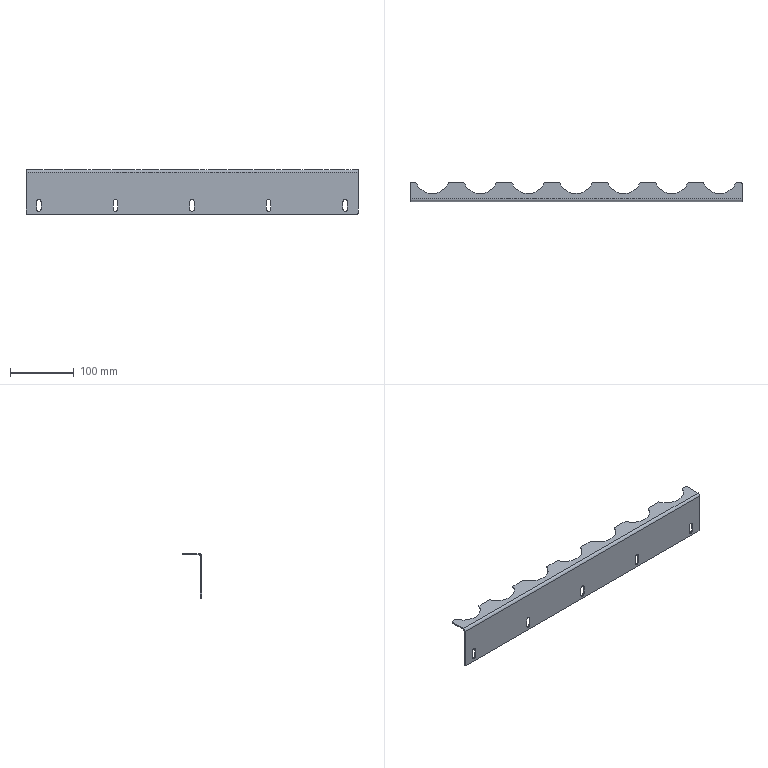Part | STEP file | 1 solid | 53 faces | box 520 x 30 x 70 mm | volume 90245 mm3 | cylinder 28 | plane 25 | commonest cylinder face diameters 7 x15 55 x7 4 x5 8 x1